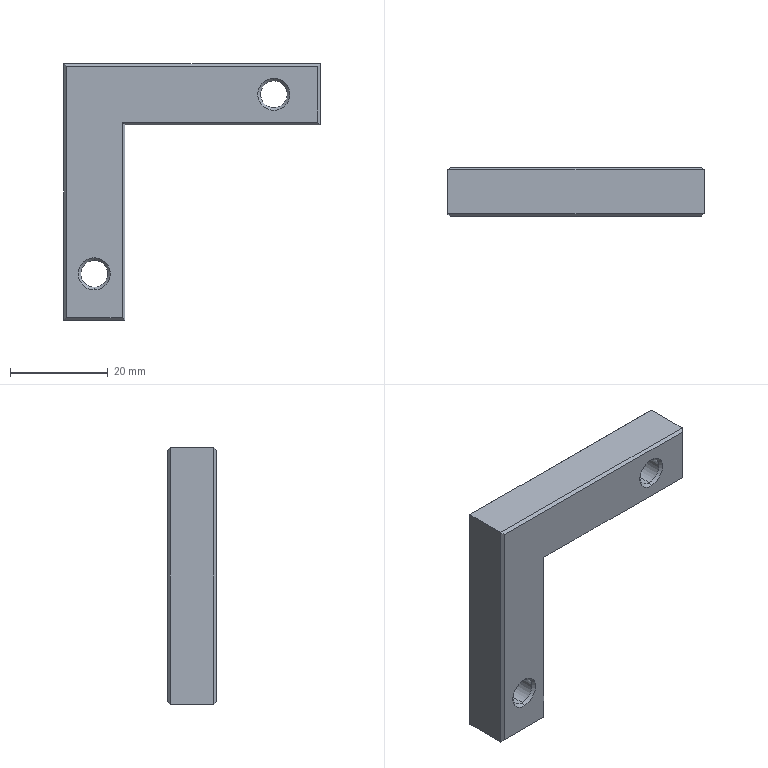Part | 1 solid | 38 faces | box 52.5 x 10 x 52.5 mm | volume 10387 mm3 | plane 22 | cone 8 | cylinder 8 | commonest cylinder face diameters 5.5 x4 10 x4
STEP:
#1=CARTESIAN_POINT('',(43.,9.46,-11.25));
#2=VERTEX_POINT('',#1);
#3=CARTESIAN_POINT('',(43.,9.46,-1.25));
#4=VERTEX_POINT('',#3);
#5=CARTESIAN_POINT('',(43.,9.46,-6.25));
#6=DIRECTION('',(0.,1.,0.));
#7=DIRECTION('',(0.,0.,-1.));
#8=AXIS2_PLACEMENT_3D('',#5,#6,#7);
#9=CIRCLE('',#8,5.);
#10=EDGE_CURVE('',#2,#4,#9,.T.);
#11=ORIENTED_EDGE('',*,*,#10,.F.);
#12=CARTESIAN_POINT('',(43.,10.,-11.79));
#13=VERTEX_POINT('',#12);
#14=CARTESIAN_POINT('',(43.,9.46,-11.25));
#15=DIRECTION('',(0.,0.7071,-0.7071));
#16=VECTOR('',#15,1000.);
#17=LINE('',#14,#16);
#18=EDGE_CURVE('',#2,#13,#17,.T.);
#19=ORIENTED_EDGE('',*,*,#18,.T.);
#20=CARTESIAN_POINT('',(43.,10.,-0.71));
#21=VERTEX_POINT('',#20);
#22=CARTESIAN_POINT('',(43.,10.,-6.25));
#23=DIRECTION('',(0.,-1.,0.));
#24=DIRECTION('',(0.,0.,-1.));
#25=AXIS2_PLACEMENT_3D('',#22,#23,#24);
#26=CIRCLE('',#25,5.54);
#27=EDGE_CURVE('',#21,#13,#26,.T.);
#28=ORIENTED_EDGE('',*,*,#27,.F.);
#29=CARTESIAN_POINT('',(43.,9.46,-1.25));
#30=DIRECTION('',(0.,0.7071,0.7071));
#31=VECTOR('',#30,1000.);
#32=LINE('',#29,#31);
#33=EDGE_CURVE('',#4,#21,#32,.T.);
#34=ORIENTED_EDGE('',*,*,#33,.F.);
#35=EDGE_LOOP('',(#11,#19,#28,#34));
#36=FACE_OUTER_BOUND('',#35,.T.);
#37=CARTESIAN_POINT('',(43.,9.46,-6.25));
#38=DIRECTION('',(0.,1.,0.));
#39=DIRECTION('',(0.,0.,1.));
#40=AXIS2_PLACEMENT_3D('',#37,#38,#39);
#41=CONICAL_SURFACE('',#40,5.,0.7854);
#42=ADVANCED_FACE('',(#36),#41,.F.);
#43=CARTESIAN_POINT('',(6.25,9.46,-48.));
#44=VERTEX_POINT('',#43);
#45=CARTESIAN_POINT('',(6.25,9.46,-38.));
#46=VERTEX_POINT('',#45);
#47=CARTESIAN_POINT('',(6.25,9.46,-43.));
#48=DIRECTION('',(0.,1.,0.));
#49=DIRECTION('',(0.,0.,-1.));
#50=AXIS2_PLACEMENT_3D('',#47,#48,#49);
#51=CIRCLE('',#50,5.);
#52=EDGE_CURVE('',#44,#46,#51,.T.);
#53=ORIENTED_EDGE('',*,*,#52,.F.);
#54=CARTESIAN_POINT('',(6.25,10.,-48.54));
#55=VERTEX_POINT('',#54);
#56=CARTESIAN_POINT('',(6.25,9.46,-48.));
#57=DIRECTION('',(0.,0.7071,-0.7071));
#58=VECTOR('',#57,1000.);
#59=LINE('',#56,#58);
#60=EDGE_CURVE('',#44,#55,#59,.T.);
#61=ORIENTED_EDGE('',*,*,#60,.T.);
#62=CARTESIAN_POINT('',(6.25,10.,-37.46));
#63=VERTEX_POINT('',#62);
#64=CARTESIAN_POINT('',(6.25,10.,-43.));
#65=DIRECTION('',(0.,-1.,0.));
#66=DIRECTION('',(0.,0.,-1.));
#67=AXIS2_PLACEMENT_3D('',#64,#65,#66);
#68=CIRCLE('',#67,5.54);
#69=EDGE_CURVE('',#63,#55,#68,.T.);
#70=ORIENTED_EDGE('',*,*,#69,.F.);
#71=CARTESIAN_POINT('',(6.25,9.46,-38.));
#72=DIRECTION('',(0.,0.7071,0.7071));
#73=VECTOR('',#72,1000.);
#74=LINE('',#71,#73);
#75=EDGE_CURVE('',#46,#63,#74,.T.);
#76=ORIENTED_EDGE('',*,*,#75,.F.);
#77=EDGE_LOOP('',(#53,#61,#70,#76));
#78=FACE_OUTER_BOUND('',#77,.T.);
#79=CARTESIAN_POINT('',(6.25,9.46,-43.));
#80=DIRECTION('',(0.,1.,0.));
#81=DIRECTION('',(0.,0.,1.));
#82=AXIS2_PLACEMENT_3D('',#79,#80,#81);
#83=CONICAL_SURFACE('',#82,5.,0.7854);
#84=ADVANCED_FACE('',(#78),#83,.F.);
#85=CARTESIAN_POINT('',(43.,0.54,-3.5));
#86=VERTEX_POINT('',#85);
#87=CARTESIAN_POINT('',(43.,0.54,-9.));
#88=VERTEX_POINT('',#87);
#89=CARTESIAN_POINT('',(43.,0.54,-6.25));
#90=DIRECTION('',(0.,-1.,0.));
#91=DIRECTION('',(0.,0.,-1.));
#92=AXIS2_PLACEMENT_3D('',#89,#90,#91);
#93=CIRCLE('',#92,2.75);
#94=EDGE_CURVE('',#86,#88,#93,.T.);
#95=ORIENTED_EDGE('',*,*,#94,.F.);
#96=CARTESIAN_POINT('',(43.,0.,-2.96));
#97=VERTEX_POINT('',#96);
#98=CARTESIAN_POINT('',(43.,0.,-2.96));
#99=DIRECTION('',(0.,-0.7071,0.7071));
#100=VECTOR('',#99,1000.);
#101=LINE('',#98,#100);
#102=EDGE_CURVE('',#86,#97,#101,.T.);
#103=ORIENTED_EDGE('',*,*,#102,.T.);
#104=CARTESIAN_POINT('',(43.,0.,-9.54));
#105=VERTEX_POINT('',#104);
#106=CARTESIAN_POINT('',(43.,0.,-6.25));
#107=DIRECTION('',(0.,1.,0.));
#108=DIRECTION('',(0.,0.,-1.));
#109=AXIS2_PLACEMENT_3D('',#106,#107,#108);
#110=CIRCLE('',#109,3.29);
#111=EDGE_CURVE('',#105,#97,#110,.T.);
#112=ORIENTED_EDGE('',*,*,#111,.F.);
#113=CARTESIAN_POINT('',(43.,0.,-9.54));
#114=DIRECTION('',(0.,-0.7071,-0.7071));
#115=VECTOR('',#114,1000.);
#116=LINE('',#113,#115);
#117=EDGE_CURVE('',#88,#105,#116,.T.);
#118=ORIENTED_EDGE('',*,*,#117,.F.);
#119=EDGE_LOOP('',(#95,#103,#112,#118));
#120=FACE_OUTER_BOUND('',#119,.T.);
#121=CARTESIAN_POINT('',(43.,0.,-6.25));
#122=DIRECTION('',(0.,-1.,0.));
#123=DIRECTION('',(0.,0.,-1.));
#124=AXIS2_PLACEMENT_3D('',#121,#122,#123);
#125=CONICAL_SURFACE('',#124,3.29,0.7854);
#126=ADVANCED_FACE('',(#120),#125,.F.);
#127=CARTESIAN_POINT('',(6.25,0.54,-40.25));
#128=VERTEX_POINT('',#127);
#129=CARTESIAN_POINT('',(6.25,0.54,-45.75));
#130=VERTEX_POINT('',#129);
#131=CARTESIAN_POINT('',(6.25,0.54,-43.));
#132=DIRECTION('',(0.,-1.,0.));
#133=DIRECTION('',(0.,0.,-1.));
#134=AXIS2_PLACEMENT_3D('',#131,#132,#133);
#135=CIRCLE('',#134,2.75);
#136=EDGE_CURVE('',#128,#130,#135,.T.);
#137=ORIENTED_EDGE('',*,*,#136,.F.);
#138=CARTESIAN_POINT('',(6.25,0.,-39.71));
#139=VERTEX_POINT('',#138);
#140=CARTESIAN_POINT('',(6.25,0.,-39.71));
#141=DIRECTION('',(0.,-0.7071,0.7071));
#142=VECTOR('',#141,1000.);
#143=LINE('',#140,#142);
#144=EDGE_CURVE('',#128,#139,#143,.T.);
#145=ORIENTED_EDGE('',*,*,#144,.T.);
#146=CARTESIAN_POINT('',(6.25,0.,-46.29));
#147=VERTEX_POINT('',#146);
#148=CARTESIAN_POINT('',(6.25,0.,-43.));
#149=DIRECTION('',(0.,1.,0.));
#150=DIRECTION('',(0.,0.,-1.));
#151=AXIS2_PLACEMENT_3D('',#148,#149,#150);
#152=CIRCLE('',#151,3.29);
#153=EDGE_CURVE('',#147,#139,#152,.T.);
#154=ORIENTED_EDGE('',*,*,#153,.F.);
#155=CARTESIAN_POINT('',(6.25,0.,-46.29));
#156=DIRECTION('',(0.,-0.7071,-0.7071));
#157=VECTOR('',#156,1000.);
#158=LINE('',#155,#157);
#159=EDGE_CURVE('',#130,#147,#158,.T.);
#160=ORIENTED_EDGE('',*,*,#159,.F.);
#161=EDGE_LOOP('',(#137,#145,#154,#160));
#162=FACE_OUTER_BOUND('',#161,.T.);
#163=CARTESIAN_POINT('',(6.25,0.,-43.));
#164=DIRECTION('',(0.,-1.,0.));
#165=DIRECTION('',(0.,0.,-1.));
#166=AXIS2_PLACEMENT_3D('',#163,#164,#165);
#167=CONICAL_SURFACE('',#166,3.29,0.7854);
#168=ADVANCED_FACE('',(#162),#167,.F.);
#169=CARTESIAN_POINT('',(43.,4.3,-11.25));
#170=VERTEX_POINT('',#169);
#171=CARTESIAN_POINT('',(43.,4.3,-1.25));
#172=VERTEX_POINT('',#171);
#173=CARTESIAN_POINT('',(43.,4.3,-6.25));
#174=DIRECTION('',(0.,1.,0.));
#175=DIRECTION('',(0.,0.,1.));
#176=AXIS2_PLACEMENT_3D('',#173,#174,#175);
#177=CIRCLE('',#176,5.);
#178=EDGE_CURVE('',#170,#172,#177,.T.);
#179=ORIENTED_EDGE('',*,*,#178,.F.);
#180=CARTESIAN_POINT('',(43.,10.,-11.25));
#181=DIRECTION('',(0.,1.,0.));
#182=VECTOR('',#181,1000.);
#183=LINE('',#180,#182);
#184=EDGE_CURVE('',#170,#2,#183,.T.);
#185=ORIENTED_EDGE('',*,*,#184,.T.);
#186=ORIENTED_EDGE('',*,*,#10,.T.);
#187=CARTESIAN_POINT('',(43.,10.,-1.25));
#188=DIRECTION('',(0.,1.,0.));
#189=VECTOR('',#188,1000.);
#190=LINE('',#187,#189);
#191=EDGE_CURVE('',#172,#4,#190,.T.);
#192=ORIENTED_EDGE('',*,*,#191,.F.);
#193=EDGE_LOOP('',(#179,#185,#186,#192));
#194=FACE_OUTER_BOUND('',#193,.T.);
#195=CARTESIAN_POINT('',(43.,10.,-6.25));
#196=DIRECTION('',(0.,1.,0.));
#197=DIRECTION('',(0.,0.,1.));
#198=AXIS2_PLACEMENT_3D('',#195,#196,#197);
#199=CYLINDRICAL_SURFACE('',#198,5.);
#200=ADVANCED_FACE('',(#194),#199,.F.);
#201=ORIENTED_EDGE('',*,*,#94,.T.);
#202=CARTESIAN_POINT('',(43.,4.3,-9.));
#203=VERTEX_POINT('',#202);
#204=CARTESIAN_POINT('',(43.,10.,-9.));
#205=DIRECTION('',(0.,1.,0.));
#206=VECTOR('',#205,1000.);
#207=LINE('',#204,#206);
#208=EDGE_CURVE('',#88,#203,#207,.T.);
#209=ORIENTED_EDGE('',*,*,#208,.T.);
#210=CARTESIAN_POINT('',(43.,4.3,-3.5));
#211=VERTEX_POINT('',#210);
#212=CARTESIAN_POINT('',(43.,4.3,-6.25));
#213=DIRECTION('',(0.,1.,0.));
#214=DIRECTION('',(0.,0.,1.));
#215=AXIS2_PLACEMENT_3D('',#212,#213,#214);
#216=CIRCLE('',#215,2.75);
#217=EDGE_CURVE('',#203,#211,#216,.T.);
#218=ORIENTED_EDGE('',*,*,#217,.T.);
#219=CARTESIAN_POINT('',(43.,10.,-3.5));
#220=DIRECTION('',(0.,1.,0.));
#221=VECTOR('',#220,1000.);
#222=LINE('',#219,#221);
#223=EDGE_CURVE('',#86,#211,#222,.T.);
#224=ORIENTED_EDGE('',*,*,#223,.F.);
#225=EDGE_LOOP('',(#201,#209,#218,#224));
#226=FACE_OUTER_BOUND('',#225,.T.);
#227=CARTESIAN_POINT('',(43.,10.,-6.25));
#228=DIRECTION('',(0.,1.,0.));
#229=DIRECTION('',(0.,0.,1.));
#230=AXIS2_PLACEMENT_3D('',#227,#228,#229);
#231=CYLINDRICAL_SURFACE('',#230,2.75);
#232=ADVANCED_FACE('',(#226),#231,.F.);
#233=CARTESIAN_POINT('',(6.25,4.3,-48.));
#234=VERTEX_POINT('',#233);
#235=CARTESIAN_POINT('',(6.25,4.3,-38.));
#236=VERTEX_POINT('',#235);
#237=CARTESIAN_POINT('',(6.25,4.3,-43.));
#238=DIRECTION('',(0.,1.,0.));
#239=DIRECTION('',(0.,0.,1.));
#240=AXIS2_PLACEMENT_3D('',#237,#238,#239);
#241=CIRCLE('',#240,5.);
#242=EDGE_CURVE('',#234,#236,#241,.T.);
#243=ORIENTED_EDGE('',*,*,#242,.F.);
#244=CARTESIAN_POINT('',(6.25,10.,-48.));
#245=DIRECTION('',(0.,1.,0.));
#246=VECTOR('',#245,1000.);
#247=LINE('',#244,#246);
#248=EDGE_CURVE('',#234,#44,#247,.T.);
#249=ORIENTED_EDGE('',*,*,#248,.T.);
#250=ORIENTED_EDGE('',*,*,#52,.T.);
#251=CARTESIAN_POINT('',(6.25,10.,-38.));
#252=DIRECTION('',(0.,1.,0.));
#253=VECTOR('',#252,1000.);
#254=LINE('',#251,#253);
#255=EDGE_CURVE('',#236,#46,#254,.T.);
#256=ORIENTED_EDGE('',*,*,#255,.F.);
#257=EDGE_LOOP('',(#243,#249,#250,#256));
#258=FACE_OUTER_BOUND('',#257,.T.);
#259=CARTESIAN_POINT('',(6.25,10.,-43.));
#260=DIRECTION('',(0.,1.,0.));
#261=DIRECTION('',(0.,0.,1.));
#262=AXIS2_PLACEMENT_3D('',#259,#260,#261);
#263=CYLINDRICAL_SURFACE('',#262,5.);
#264=ADVANCED_FACE('',(#258),#263,.F.);
#265=ORIENTED_EDGE('',*,*,#136,.T.);
#266=CARTESIAN_POINT('',(6.25,4.3,-45.75));
#267=VERTEX_POINT('',#266);
#268=CARTESIAN_POINT('',(6.25,10.,-45.75));
#269=DIRECTION('',(0.,1.,0.));
#270=VECTOR('',#269,1000.);
#271=LINE('',#268,#270);
#272=EDGE_CURVE('',#130,#267,#271,.T.);
#273=ORIENTED_EDGE('',*,*,#272,.T.);
#274=CARTESIAN_POINT('',(6.25,4.3,-40.25));
#275=VERTEX_POINT('',#274);
#276=CARTESIAN_POINT('',(6.25,4.3,-43.));
#277=DIRECTION('',(0.,1.,0.));
#278=DIRECTION('',(0.,0.,1.));
#279=AXIS2_PLACEMENT_3D('',#276,#277,#278);
#280=CIRCLE('',#279,2.75);
#281=EDGE_CURVE('',#267,#275,#280,.T.);
#282=ORIENTED_EDGE('',*,*,#281,.T.);
#283=CARTESIAN_POINT('',(6.25,10.,-40.25));
#284=DIRECTION('',(0.,1.,0.));
#285=VECTOR('',#284,1000.);
#286=LINE('',#283,#285);
#287=EDGE_CURVE('',#128,#275,#286,.T.);
#288=ORIENTED_EDGE('',*,*,#287,.F.);
#289=EDGE_LOOP('',(#265,#273,#282,#288));
#290=FACE_OUTER_BOUND('',#289,.T.);
#291=CARTESIAN_POINT('',(6.25,10.,-43.));
#292=DIRECTION('',(0.,1.,0.));
#293=DIRECTION('',(0.,0.,1.));
#294=AXIS2_PLACEMENT_3D('',#291,#292,#293);
#295=CYLINDRICAL_SURFACE('',#294,2.75);
#296=ADVANCED_FACE('',(#290),#295,.F.);
#297=CARTESIAN_POINT('',(0.,9.46,0.));
#298=VERTEX_POINT('',#297);
#299=CARTESIAN_POINT('',(0.,0.54,0.));
#300=VERTEX_POINT('',#299);
#301=CARTESIAN_POINT('',(0.,10.,0.));
#302=DIRECTION('',(0.,-1.,0.));
#303=VECTOR('',#302,1000.);
#304=LINE('',#301,#303);
#305=EDGE_CURVE('',#298,#300,#304,.T.);
#306=ORIENTED_EDGE('',*,*,#305,.T.);
#307=CARTESIAN_POINT('',(52.5,0.54,0.));
#308=VERTEX_POINT('',#307);
#309=CARTESIAN_POINT('',(52.5,0.54,0.));
#310=DIRECTION('',(1.,0.,0.));
#311=VECTOR('',#310,1000.);
#312=LINE('',#309,#311);
#313=EDGE_CURVE('',#300,#308,#312,.T.);
#314=ORIENTED_EDGE('',*,*,#313,.T.);
#315=CARTESIAN_POINT('',(52.5,9.46,0.));
#316=VERTEX_POINT('',#315);
#317=CARTESIAN_POINT('',(52.5,10.,0.));
#318=DIRECTION('',(0.,-1.,0.));
#319=VECTOR('',#318,1000.);
#320=LINE('',#317,#319);
#321=EDGE_CURVE('',#316,#308,#320,.T.);
#322=ORIENTED_EDGE('',*,*,#321,.F.);
#323=CARTESIAN_POINT('',(52.5,9.46,0.));
#324=DIRECTION('',(-1.,0.,0.));
#325=VECTOR('',#324,1000.);
#326=LINE('',#323,#325);
#327=EDGE_CURVE('',#316,#298,#326,.T.);
#328=ORIENTED_EDGE('',*,*,#327,.T.);
#329=EDGE_LOOP('',(#306,#314,#322,#328));
#330=FACE_OUTER_BOUND('',#329,.T.);
#331=CARTESIAN_POINT('',(52.5,10.,0.));
#332=DIRECTION('',(0.,0.,-1.));
#333=DIRECTION('',(-1.,0.,0.));
#334=AXIS2_PLACEMENT_3D('',#331,#332,#333);
#335=PLANE('',#334);
#336=ADVANCED_FACE('',(#330),#335,.F.);
#337=ORIENTED_EDGE('',*,*,#321,.T.);
#338=CARTESIAN_POINT('',(52.5,0.54,-12.5));
#339=VERTEX_POINT('',#338);
#340=CARTESIAN_POINT('',(52.5,0.54,-12.5));
#341=DIRECTION('',(0.,0.,-1.));
#342=VECTOR('',#341,1000.);
#343=LINE('',#340,#342);
#344=EDGE_CURVE('',#308,#339,#343,.T.);
#345=ORIENTED_EDGE('',*,*,#344,.T.);
#346=CARTESIAN_POINT('',(52.5,9.46,-12.5));
#347=VERTEX_POINT('',#346);
#348=CARTESIAN_POINT('',(52.5,10.,-12.5));
#349=DIRECTION('',(0.,-1.,0.));
#350=VECTOR('',#349,1000.);
#351=LINE('',#348,#350);
#352=EDGE_CURVE('',#347,#339,#351,.T.);
#353=ORIENTED_EDGE('',*,*,#352,.F.);
#354=CARTESIAN_POINT('',(52.5,9.46,-12.5));
#355=DIRECTION('',(0.,0.,1.));
#356=VECTOR('',#355,1000.);
#357=LINE('',#354,#356);
#358=EDGE_CURVE('',#347,#316,#357,.T.);
#359=ORIENTED_EDGE('',*,*,#358,.T.);
#360=EDGE_LOOP('',(#337,#345,#353,#359));
#361=FACE_OUTER_BOUND('',#360,.T.);
#362=CARTESIAN_POINT('',(52.5,10.,-12.5));
#363=DIRECTION('',(-1.,0.,0.));
#364=DIRECTION('',(0.,0.,1.));
#365=AXIS2_PLACEMENT_3D('',#362,#363,#364);
#366=PLANE('',#365);
#367=ADVANCED_FACE('',(#361),#366,.F.);
#368=ORIENTED_EDGE('',*,*,#352,.T.);
#369=CARTESIAN_POINT('',(12.5,0.54,-12.5));
#370=VERTEX_POINT('',#369);
#371=CARTESIAN_POINT('',(12.5,0.54,-12.5));
#372=DIRECTION('',(-1.,0.,0.));
#373=VECTOR('',#372,1000.);
#374=LINE('',#371,#373);
#375=EDGE_CURVE('',#339,#370,#374,.T.);
#376=ORIENTED_EDGE('',*,*,#375,.T.);
#377=CARTESIAN_POINT('',(12.5,9.46,-12.5));
#378=VERTEX_POINT('',#377);
#379=CARTESIAN_POINT('',(12.5,10.,-12.5));
#380=DIRECTION('',(0.,-1.,0.));
#381=VECTOR('',#380,1000.);
#382=LINE('',#379,#381);
#383=EDGE_CURVE('',#378,#370,#382,.T.);
#384=ORIENTED_EDGE('',*,*,#383,.F.);
#385=CARTESIAN_POINT('',(12.5,9.46,-12.5));
#386=DIRECTION('',(1.,0.,0.));
#387=VECTOR('',#386,1000.);
#388=LINE('',#385,#387);
#389=EDGE_CURVE('',#378,#347,#388,.T.);
#390=ORIENTED_EDGE('',*,*,#389,.T.);
#391=EDGE_LOOP('',(#368,#376,#384,#390));
#392=FACE_OUTER_BOUND('',#391,.T.);
#393=CARTESIAN_POINT('',(12.5,10.,-12.5));
#394=DIRECTION('',(0.,0.,1.));
#395=DIRECTION('',(1.,0.,0.));
#396=AXIS2_PLACEMENT_3D('',#393,#394,#395);
#397=PLANE('',#396);
#398=ADVANCED_FACE('',(#392),#397,.F.);
#399=ORIENTED_EDGE('',*,*,#383,.T.);
#400=CARTESIAN_POINT('',(12.5,0.54,-52.5));
#401=VERTEX_POINT('',#400);
#402=CARTESIAN_POINT('',(12.5,0.54,-52.5));
#403=DIRECTION('',(0.,0.,-1.));
#404=VECTOR('',#403,1000.);
#405=LINE('',#402,#404);
#406=EDGE_CURVE('',#370,#401,#405,.T.);
#407=ORIENTED_EDGE('',*,*,#406,.T.);
#408=CARTESIAN_POINT('',(12.5,9.46,-52.5));
#409=VERTEX_POINT('',#408);
#410=CARTESIAN_POINT('',(12.5,10.,-52.5));
#411=DIRECTION('',(0.,-1.,0.));
#412=VECTOR('',#411,1000.);
#413=LINE('',#410,#412);
#414=EDGE_CURVE('',#409,#401,#413,.T.);
#415=ORIENTED_EDGE('',*,*,#414,.F.);
#416=CARTESIAN_POINT('',(12.5,9.46,-52.5));
#417=DIRECTION('',(0.,0.,1.));
#418=VECTOR('',#417,1000.);
#419=LINE('',#416,#418);
#420=EDGE_CURVE('',#409,#378,#419,.T.);
#421=ORIENTED_EDGE('',*,*,#420,.T.);
#422=EDGE_LOOP('',(#399,#407,#415,#421));
#423=FACE_OUTER_BOUND('',#422,.T.);
#424=CARTESIAN_POINT('',(12.5,10.,-52.5));
#425=DIRECTION('',(-1.,0.,0.));
#426=DIRECTION('',(0.,0.,1.));
#427=AXIS2_PLACEMENT_3D('',#424,#425,#426);
#428=PLANE('',#427);
#429=ADVANCED_FACE('',(#423),#428,.F.);
#430=ORIENTED_EDGE('',*,*,#414,.T.);
#431=CARTESIAN_POINT('',(0.,0.54,-52.5));
#432=VERTEX_POINT('',#431);
#433=CARTESIAN_POINT('',(0.,0.54,-52.5));
#434=DIRECTION('',(-1.,0.,0.));
#435=VECTOR('',#434,1000.);
#436=LINE('',#433,#435);
#437=EDGE_CURVE('',#401,#432,#436,.T.);
#438=ORIENTED_EDGE('',*,*,#437,.T.);
#439=CARTESIAN_POINT('',(0.,9.46,-52.5));
#440=VERTEX_POINT('',#439);
#441=CARTESIAN_POINT('',(0.,10.,-52.5));
#442=DIRECTION('',(0.,-1.,0.));
#443=VECTOR('',#442,1000.);
#444=LINE('',#441,#443);
#445=EDGE_CURVE('',#440,#432,#444,.T.);
#446=ORIENTED_EDGE('',*,*,#445,.F.);
#447=CARTESIAN_POINT('',(0.,9.46,-52.5));
#448=DIRECTION('',(1.,0.,0.));
#449=VECTOR('',#448,1000.);
#450=LINE('',#447,#449);
#451=EDGE_CURVE('',#440,#409,#450,.T.);
#452=ORIENTED_EDGE('',*,*,#451,.T.);
#453=EDGE_LOOP('',(#430,#438,#446,#452));
#454=FACE_OUTER_BOUND('',#453,.T.);
#455=CARTESIAN_POINT('',(0.,10.,-52.5));
#456=DIRECTION('',(0.,0.,1.));
#457=DIRECTION('',(1.,0.,0.));
#458=AXIS2_PLACEMENT_3D('',#455,#456,#457);
#459=PLANE('',#458);
#460=ADVANCED_FACE('',(#454),#459,.F.);
#461=ORIENTED_EDGE('',*,*,#445,.T.);
#462=CARTESIAN_POINT('',(0.,0.54,0.));
#463=DIRECTION('',(0.,0.,1.));
#464=VECTOR('',#463,1000.);
#465=LINE('',#462,#464);
#466=EDGE_CURVE('',#432,#300,#465,.T.);
#467=ORIENTED_EDGE('',*,*,#466,.T.);
#468=ORIENTED_EDGE('',*,*,#305,.F.);
#469=CARTESIAN_POINT('',(0.,9.46,0.));
#470=DIRECTION('',(0.,0.,-1.));
#471=VECTOR('',#470,1000.);
#472=LINE('',#469,#471);
#473=EDGE_CURVE('',#298,#440,#472,.T.);
#474=ORIENTED_EDGE('',*,*,#473,.T.);
#475=EDGE_LOOP('',(#461,#467,#468,#474));
#476=FACE_OUTER_BOUND('',#475,.T.);
#477=CARTESIAN_POINT('',(0.,10.,0.));
#478=DIRECTION('',(1.,0.,0.));
#479=DIRECTION('',(0.,0.,-1.));
#480=AXIS2_PLACEMENT_3D('',#477,#478,#479);
#481=PLANE('',#480);
#482=ADVANCED_FACE('',(#476),#481,.F.);
#483=CARTESIAN_POINT('',(11.96,10.,-51.96));
#484=VERTEX_POINT('',#483);
#485=CARTESIAN_POINT('',(0.54,10.,-51.96));
#486=VERTEX_POINT('',#485);
#487=CARTESIAN_POINT('',(0.,10.,-51.96));
#488=DIRECTION('',(-1.,0.,0.));
#489=VECTOR('',#488,1000.);
#490=LINE('',#487,#489);
#491=EDGE_CURVE('',#484,#486,#490,.T.);
#492=ORIENTED_EDGE('',*,*,#491,.T.);
#493=CARTESIAN_POINT('',(0.54,10.,-0.54));
#494=VERTEX_POINT('',#493);
#495=CARTESIAN_POINT('',(0.54,10.,0.));
#496=DIRECTION('',(0.,0.,1.));
#497=VECTOR('',#496,1000.);
#498=LINE('',#495,#497);
#499=EDGE_CURVE('',#486,#494,#498,.T.);
#500=ORIENTED_EDGE('',*,*,#499,.T.);
#501=CARTESIAN_POINT('',(51.96,10.,-0.54));
#502=VERTEX_POINT('',#501);
#503=CARTESIAN_POINT('',(0.,10.,-0.54));
#504=DIRECTION('',(1.,0.,0.));
#505=VECTOR('',#504,1000.);
#506=LINE('',#503,#505);
#507=EDGE_CURVE('',#494,#502,#506,.T.);
#508=ORIENTED_EDGE('',*,*,#507,.T.);
#509=CARTESIAN_POINT('',(51.96,10.,-11.96));
#510=VERTEX_POINT('',#509);
#511=CARTESIAN_POINT('',(51.96,10.,0.));
#512=DIRECTION('',(0.,0.,-1.));
#513=VECTOR('',#512,1000.);
#514=LINE('',#511,#513);
#515=EDGE_CURVE('',#502,#510,#514,.T.);
#516=ORIENTED_EDGE('',*,*,#515,.T.);
#517=CARTESIAN_POINT('',(11.96,10.,-11.96));
#518=VERTEX_POINT('',#517);
#519=CARTESIAN_POINT('',(0.,10.,-11.96));
#520=DIRECTION('',(-1.,0.,0.));
#521=VECTOR('',#520,1000.);
#522=LINE('',#519,#521);
#523=EDGE_CURVE('',#510,#518,#522,.T.);
#524=ORIENTED_EDGE('',*,*,#523,.T.);
#525=CARTESIAN_POINT('',(11.96,10.,0.));
#526=DIRECTION('',(0.,0.,-1.));
#527=VECTOR('',#526,1000.);
#528=LINE('',#525,#527);
#529=EDGE_CURVE('',#518,#484,#528,.T.);
#530=ORIENTED_EDGE('',*,*,#529,.T.);
#531=EDGE_LOOP('',(#492,#500,#508,#516,#524,#530));
#532=FACE_OUTER_BOUND('',#531,.T.);
#533=ORIENTED_EDGE('',*,*,#69,.T.);
#534=CARTESIAN_POINT('',(6.25,10.,-43.));
#535=DIRECTION('',(0.,-1.,0.));
#536=DIRECTION('',(0.,0.,-1.));
#537=AXIS2_PLACEMENT_3D('',#534,#535,#536);
#538=CIRCLE('',#537,5.54);
#539=EDGE_CURVE('',#55,#63,#538,.T.);
#540=ORIENTED_EDGE('',*,*,#539,.T.);
#541=EDGE_LOOP('',(#533,#540));
#542=FACE_BOUND('',#541,.T.);
#543=ORIENTED_EDGE('',*,*,#27,.T.);
#544=CARTESIAN_POINT('',(43.,10.,-6.25));
#545=DIRECTION('',(0.,-1.,0.));
#546=DIRECTION('',(0.,0.,-1.));
#547=AXIS2_PLACEMENT_3D('',#544,#545,#546);
#548=CIRCLE('',#547,5.54);
#549=EDGE_CURVE('',#13,#21,#548,.T.);
#550=ORIENTED_EDGE('',*,*,#549,.T.);
#551=EDGE_LOOP('',(#543,#550));
#552=FACE_BOUND('',#551,.T.);
#553=CARTESIAN_POINT('',(0.,10.,0.));
#554=DIRECTION('',(0.,-1.,0.));
#555=DIRECTION('',(0.,0.,-1.));
#556=AXIS2_PLACEMENT_3D('',#553,#554,#555);
#557=PLANE('',#556);
#558=ADVANCED_FACE('',(#532,#542,#552),#557,.F.);
#559=CARTESIAN_POINT('',(11.96,0.,-11.96));
#560=VERTEX_POINT('',#559);
#561=CARTESIAN_POINT('',(51.96,0.,-11.96));
#562=VERTEX_POINT('',#561);
#563=CARTESIAN_POINT('',(52.5,0.,-11.96));
#564=DIRECTION('',(1.,0.,0.));
#565=VECTOR('',#564,1000.);
#566=LINE('',#563,#565);
#567=EDGE_CURVE('',#560,#562,#566,.T.);
#568=ORIENTED_EDGE('',*,*,#567,.T.);
#569=CARTESIAN_POINT('',(51.96,0.,-0.54));
#570=VERTEX_POINT('',#569);
#571=CARTESIAN_POINT('',(51.96,0.,0.));
#572=DIRECTION('',(0.,0.,1.));
#573=VECTOR('',#572,1000.);
#574=LINE('',#571,#573);
#575=EDGE_CURVE('',#562,#570,#574,.T.);
#576=ORIENTED_EDGE('',*,*,#575,.T.);
#577=CARTESIAN_POINT('',(0.54,0.,-0.54));
#578=VERTEX_POINT('',#577);
#579=CARTESIAN_POINT('',(0.,0.,-0.54));
#580=DIRECTION('',(-1.,0.,0.));
#581=VECTOR('',#580,1000.);
#582=LINE('',#579,#581);
#583=EDGE_CURVE('',#570,#578,#582,.T.);
#584=ORIENTED_EDGE('',*,*,#583,.T.);
#585=CARTESIAN_POINT('',(0.54,0.,-51.96));
#586=VERTEX_POINT('',#585);
#587=CARTESIAN_POINT('',(0.54,0.,-52.5));
#588=DIRECTION('',(0.,0.,-1.));
#589=VECTOR('',#588,1000.);
#590=LINE('',#587,#589);
#591=EDGE_CURVE('',#578,#586,#590,.T.);
#592=ORIENTED_EDGE('',*,*,#591,.T.);
#593=CARTESIAN_POINT('',(11.96,0.,-51.96));
#594=VERTEX_POINT('',#593);
#595=CARTESIAN_POINT('',(12.5,0.,-51.96));
#596=DIRECTION('',(1.,0.,0.));
#597=VECTOR('',#596,1000.);
#598=LINE('',#595,#597);
#599=EDGE_CURVE('',#586,#594,#598,.T.);
#600=ORIENTED_EDGE('',*,*,#599,.T.);
#601=CARTESIAN_POINT('',(11.96,0.,-12.5));
#602=DIRECTION('',(0.,0.,1.));
#603=VECTOR('',#602,1000.);
#604=LINE('',#601,#603);
#605=EDGE_CURVE('',#594,#560,#604,.T.);
#606=ORIENTED_EDGE('',*,*,#605,.T.);
#607=EDGE_LOOP('',(#568,#576,#584,#592,#600,#606));
#608=FACE_OUTER_BOUND('',#607,.T.);
#609=ORIENTED_EDGE('',*,*,#153,.T.);
#610=CARTESIAN_POINT('',(6.25,0.,-43.));
#611=DIRECTION('',(0.,1.,0.));
#612=DIRECTION('',(0.,0.,-1.));
#613=AXIS2_PLACEMENT_3D('',#610,#611,#612);
#614=CIRCLE('',#613,3.29);
#615=EDGE_CURVE('',#139,#147,#614,.T.);
#616=ORIENTED_EDGE('',*,*,#615,.T.);
#617=EDGE_LOOP('',(#609,#616));
#618=FACE_BOUND('',#617,.T.);
#619=ORIENTED_EDGE('',*,*,#111,.T.);
#620=CARTESIAN_POINT('',(43.,0.,-6.25));
#621=DIRECTION('',(0.,1.,0.));
#622=DIRECTION('',(0.,0.,-1.));
#623=AXIS2_PLACEMENT_3D('',#620,#621,#622);
#624=CIRCLE('',#623,3.29);
#625=EDGE_CURVE('',#97,#105,#624,.T.);
#626=ORIENTED_EDGE('',*,*,#625,.T.);
#627=EDGE_LOOP('',(#619,#626));
#628=FACE_BOUND('',#627,.T.);
#629=CARTESIAN_POINT('',(0.,0.,0.));
#630=DIRECTION('',(0.,-1.,0.));
#631=DIRECTION('',(0.,0.,-1.));
#632=AXIS2_PLACEMENT_3D('',#629,#630,#631);
#633=PLANE('',#632);
#634=ADVANCED_FACE('',(#608,#618,#628),#633,.T.);
#635=ORIENTED_EDGE('',*,*,#272,.F.);
#636=CARTESIAN_POINT('',(6.25,0.54,-43.));
#637=DIRECTION('',(0.,-1.,0.));
#638=DIRECTION('',(0.,0.,-1.));
#639=AXIS2_PLACEMENT_3D('',#636,#637,#638);
#640=CIRCLE('',#639,2.75);
#641=EDGE_CURVE('',#130,#128,#640,.T.);
#642=ORIENTED_EDGE('',*,*,#641,.T.);
#643=ORIENTED_EDGE('',*,*,#287,.T.);
#644=CARTESIAN_POINT('',(6.25,4.3,-43.));
#645=DIRECTION('',(0.,1.,0.));
#646=DIRECTION('',(0.,0.,1.));
#647=AXIS2_PLACEMENT_3D('',#644,#645,#646);
#648=CIRCLE('',#647,2.75);
#649=EDGE_CURVE('',#275,#267,#648,.T.);
#650=ORIENTED_EDGE('',*,*,#649,.T.);
#651=EDGE_LOOP('',(#635,#642,#643,#650));
#652=FACE_OUTER_BOUND('',#651,.T.);
#653=CARTESIAN_POINT('',(6.25,10.,-43.));
#654=DIRECTION('',(0.,1.,0.));
#655=DIRECTION('',(0.,0.,1.));
#656=AXIS2_PLACEMENT_3D('',#653,#654,#655);
#657=CYLINDRICAL_SURFACE('',#656,2.75);
#658=ADVANCED_FACE('',(#652),#657,.F.);
#659=ORIENTED_EDGE('',*,*,#649,.F.);
#660=ORIENTED_EDGE('',*,*,#281,.F.);
#661=EDGE_LOOP('',(#659,#660));
#662=FACE_BOUND('',#661,.T.);
#663=CARTESIAN_POINT('',(6.25,4.3,-43.));
#664=DIRECTION('',(0.,1.,0.));
#665=DIRECTION('',(0.,0.,1.));
#666=AXIS2_PLACEMENT_3D('',#663,#664,#665);
#667=CIRCLE('',#666,5.);
#668=EDGE_CURVE('',#236,#234,#667,.T.);
#669=ORIENTED_EDGE('',*,*,#668,.T.);
#670=ORIENTED_EDGE('',*,*,#242,.T.);
#671=EDGE_LOOP('',(#669,#670));
#672=FACE_OUTER_BOUND('',#671,.T.);
#673=CARTESIAN_POINT('',(9.,4.3,-43.));
#674=DIRECTION('',(0.,-1.,0.));
#675=DIRECTION('',(0.,0.,-1.));
#676=AXIS2_PLACEMENT_3D('',#673,#674,#675);
#677=PLANE('',#676);
#678=ADVANCED_FACE('',(#662,#672),#677,.F.);
#679=ORIENTED_EDGE('',*,*,#248,.F.);
#680=ORIENTED_EDGE('',*,*,#668,.F.);
#681=ORIENTED_EDGE('',*,*,#255,.T.);
#682=CARTESIAN_POINT('',(6.25,9.46,-43.));
#683=DIRECTION('',(0.,1.,0.));
#684=DIRECTION('',(0.,0.,-1.));
#685=AXIS2_PLACEMENT_3D('',#682,#683,#684);
#686=CIRCLE('',#685,5.);
#687=EDGE_CURVE('',#46,#44,#686,.T.);
#688=ORIENTED_EDGE('',*,*,#687,.T.);
#689=EDGE_LOOP('',(#679,#680,#681,#688));
#690=FACE_OUTER_BOUND('',#689,.T.);
#691=CARTESIAN_POINT('',(6.25,10.,-43.));
#692=DIRECTION('',(0.,1.,0.));
#693=DIRECTION('',(0.,0.,1.));
#694=AXIS2_PLACEMENT_3D('',#691,#692,#693);
#695=CYLINDRICAL_SURFACE('',#694,5.);
#696=ADVANCED_FACE('',(#690),#695,.F.);
#697=ORIENTED_EDGE('',*,*,#208,.F.);
#698=CARTESIAN_POINT('',(43.,0.54,-6.25));
#699=DIRECTION('',(0.,-1.,0.));
#700=DIRECTION('',(0.,0.,-1.));
#701=AXIS2_PLACEMENT_3D('',#698,#699,#700);
#702=CIRCLE('',#701,2.75);
#703=EDGE_CURVE('',#88,#86,#702,.T.);
#704=ORIENTED_EDGE('',*,*,#703,.T.);
#705=ORIENTED_EDGE('',*,*,#223,.T.);
#706=CARTESIAN_POINT('',(43.,4.3,-6.25));
#707=DIRECTION('',(0.,1.,0.));
#708=DIRECTION('',(0.,0.,1.));
#709=AXIS2_PLACEMENT_3D('',#706,#707,#708);
#710=CIRCLE('',#709,2.75);
#711=EDGE_CURVE('',#211,#203,#710,.T.);
#712=ORIENTED_EDGE('',*,*,#711,.T.);
#713=EDGE_LOOP('',(#697,#704,#705,#712));
#714=FACE_OUTER_BOUND('',#713,.T.);
#715=CARTESIAN_POINT('',(43.,10.,-6.25));
#716=DIRECTION('',(0.,1.,0.));
#717=DIRECTION('',(0.,0.,1.));
#718=AXIS2_PLACEMENT_3D('',#715,#716,#717);
#719=CYLINDRICAL_SURFACE('',#718,2.75);
#720=ADVANCED_FACE('',(#714),#719,.F.);
#721=ORIENTED_EDGE('',*,*,#711,.F.);
#722=ORIENTED_EDGE('',*,*,#217,.F.);
#723=EDGE_LOOP('',(#721,#722));
#724=FACE_BOUND('',#723,.T.);
#725=CARTESIAN_POINT('',(43.,4.3,-6.25));
#726=DIRECTION('',(0.,1.,0.));
#727=DIRECTION('',(0.,0.,1.));
#728=AXIS2_PLACEMENT_3D('',#725,#726,#727);
#729=CIRCLE('',#728,5.);
#730=EDGE_CURVE('',#172,#170,#729,.T.);
#731=ORIENTED_EDGE('',*,*,#730,.T.);
#732=ORIENTED_EDGE('',*,*,#178,.T.);
#733=EDGE_LOOP('',(#731,#732));
#734=FACE_OUTER_BOUND('',#733,.T.);
#735=CARTESIAN_POINT('',(45.75,4.3,-6.25));
#736=DIRECTION('',(0.,-1.,0.));
#737=DIRECTION('',(0.,0.,-1.));
#738=AXIS2_PLACEMENT_3D('',#735,#736,#737);
#739=PLANE('',#738);
#740=ADVANCED_FACE('',(#724,#734),#739,.F.);
#741=ORIENTED_EDGE('',*,*,#184,.F.);
#742=ORIENTED_EDGE('',*,*,#730,.F.);
#743=ORIENTED_EDGE('',*,*,#191,.T.);
#744=CARTESIAN_POINT('',(43.,9.46,-6.25));
#745=DIRECTION('',(0.,1.,0.));
#746=DIRECTION('',(0.,0.,-1.));
#747=AXIS2_PLACEMENT_3D('',#744,#745,#746);
#748=CIRCLE('',#747,5.);
#749=EDGE_CURVE('',#4,#2,#748,.T.);
#750=ORIENTED_EDGE('',*,*,#749,.T.);
#751=EDGE_LOOP('',(#741,#742,#743,#750));
#752=FACE_OUTER_BOUND('',#751,.T.);
#753=CARTESIAN_POINT('',(43.,10.,-6.25));
#754=DIRECTION('',(0.,1.,0.));
#755=DIRECTION('',(0.,0.,1.));
#756=AXIS2_PLACEMENT_3D('',#753,#754,#755);
#757=CYLINDRICAL_SURFACE('',#756,5.);
#758=ADVANCED_FACE('',(#752),#757,.F.);
#759=CARTESIAN_POINT('',(8.333,-3.627,-48.333));
#760=DIRECTION('',(0.5774,0.5774,-0.5774));
#761=VECTOR('',#760,1000.);
#762=LINE('',#759,#761);
#763=EDGE_CURVE('',#594,#401,#762,.T.);
#764=ORIENTED_EDGE('',*,*,#763,.F.);
#765=ORIENTED_EDGE('',*,*,#599,.F.);
#766=CARTESIAN_POINT('',(17.5,-16.96,-35.));
#767=DIRECTION('',(0.5774,-0.5774,0.5774));
#768=VECTOR('',#767,1000.);
#769=LINE('',#766,#768);
#770=EDGE_CURVE('',#432,#586,#769,.T.);
#771=ORIENTED_EDGE('',*,*,#770,.F.);
#772=ORIENTED_EDGE('',*,*,#437,.F.);
#773=EDGE_LOOP('',(#764,#765,#771,#772));
#774=FACE_OUTER_BOUND('',#773,.T.);
#775=CARTESIAN_POINT('',(0.,0.54,-52.5));
#776=DIRECTION('',(0.,-0.7071,-0.7071));
#777=DIRECTION('',(1.,0.,0.));
#778=AXIS2_PLACEMENT_3D('',#775,#776,#777);
#779=PLANE('',#778);
#780=ADVANCED_FACE('',(#774),#779,.T.);
#781=ORIENTED_EDGE('',*,*,#770,.T.);
#782=ORIENTED_EDGE('',*,*,#591,.F.);
#783=CARTESIAN_POINT('',(17.5,-16.96,-17.5));
#784=DIRECTION('',(0.5774,-0.5774,-0.5774));
#785=VECTOR('',#784,1000.);
#786=LINE('',#783,#785);
#787=EDGE_CURVE('',#300,#578,#786,.T.);
#788=ORIENTED_EDGE('',*,*,#787,.F.);
#789=ORIENTED_EDGE('',*,*,#466,.F.);
#790=EDGE_LOOP('',(#781,#782,#788,#789));
#791=FACE_OUTER_BOUND('',#790,.T.);
#792=CARTESIAN_POINT('',(0.,0.54,0.));
#793=DIRECTION('',(-0.7071,-0.7071,0.));
#794=DIRECTION('',(0.,0.,-1.));
#795=AXIS2_PLACEMENT_3D('',#792,#793,#794);
#796=PLANE('',#795);
#797=ADVANCED_FACE('',(#791),#796,.T.);
#798=ORIENTED_EDGE('',*,*,#763,.T.);
#799=ORIENTED_EDGE('',*,*,#406,.F.);
#800=CARTESIAN_POINT('',(12.5,0.54,-12.5));
#801=DIRECTION('',(0.5774,0.5774,-0.5774));
#802=VECTOR('',#801,1000.);
#803=LINE('',#800,#802);
#804=EDGE_CURVE('',#560,#370,#803,.T.);
#805=ORIENTED_EDGE('',*,*,#804,.F.);
#806=ORIENTED_EDGE('',*,*,#605,.F.);
#807=EDGE_LOOP('',(#798,#799,#805,#806));
#808=FACE_OUTER_BOUND('',#807,.T.);
#809=CARTESIAN_POINT('',(12.5,0.54,-52.5));
#810=DIRECTION('',(0.7071,-0.7071,0.));
#811=DIRECTION('',(0.,0.,1.));
#812=AXIS2_PLACEMENT_3D('',#809,#810,#811);
#813=PLANE('',#812);
#814=ADVANCED_FACE('',(#808),#813,.T.);
#815=ORIENTED_EDGE('',*,*,#787,.T.);
#816=ORIENTED_EDGE('',*,*,#583,.F.);
#817=CARTESIAN_POINT('',(52.5,0.54,0.));
#818=DIRECTION('',(-0.5774,-0.5774,-0.5774));
#819=VECTOR('',#818,1000.);
#820=LINE('',#817,#819);
#821=EDGE_CURVE('',#308,#570,#820,.T.);
#822=ORIENTED_EDGE('',*,*,#821,.F.);
#823=ORIENTED_EDGE('',*,*,#313,.F.);
#824=EDGE_LOOP('',(#815,#816,#822,#823));
#825=FACE_OUTER_BOUND('',#824,.T.);
#826=CARTESIAN_POINT('',(52.5,0.54,0.));
#827=DIRECTION('',(0.,-0.7071,0.7071));
#828=DIRECTION('',(-1.,0.,0.));
#829=AXIS2_PLACEMENT_3D('',#826,#827,#828);
#830=PLANE('',#829);
#831=ADVANCED_FACE('',(#825),#830,.T.);
#832=ORIENTED_EDGE('',*,*,#804,.T.);
#833=ORIENTED_EDGE('',*,*,#375,.F.);
#834=CARTESIAN_POINT('',(39.167,-12.793,0.8333));
#835=DIRECTION('',(0.5774,0.5774,-0.5774));
#836=VECTOR('',#835,1000.);
#837=LINE('',#834,#836);
#838=EDGE_CURVE('',#562,#339,#837,.T.);
#839=ORIENTED_EDGE('',*,*,#838,.F.);
#840=ORIENTED_EDGE('',*,*,#567,.F.);
#841=EDGE_LOOP('',(#832,#833,#839,#840));
#842=FACE_OUTER_BOUND('',#841,.T.);
#843=CARTESIAN_POINT('',(12.5,0.54,-12.5));
#844=DIRECTION('',(0.,-0.7071,-0.7071));
#845=DIRECTION('',(1.,0.,0.));
#846=AXIS2_PLACEMENT_3D('',#843,#844,#845);
#847=PLANE('',#846);
#848=ADVANCED_FACE('',(#842),#847,.T.);
#849=ORIENTED_EDGE('',*,*,#821,.T.);
#850=ORIENTED_EDGE('',*,*,#575,.F.);
#851=ORIENTED_EDGE('',*,*,#838,.T.);
#852=ORIENTED_EDGE('',*,*,#344,.F.);
#853=EDGE_LOOP('',(#849,#850,#851,#852));
#854=FACE_OUTER_BOUND('',#853,.T.);
#855=CARTESIAN_POINT('',(52.5,0.54,-12.5));
#856=DIRECTION('',(0.7071,-0.7071,0.));
#857=DIRECTION('',(0.,0.,1.));
#858=AXIS2_PLACEMENT_3D('',#855,#856,#857);
#859=PLANE('',#858);
#860=ADVANCED_FACE('',(#854),#859,.T.);
#861=ORIENTED_EDGE('',*,*,#144,.F.);
#862=ORIENTED_EDGE('',*,*,#641,.F.);
#863=ORIENTED_EDGE('',*,*,#159,.T.);
#864=ORIENTED_EDGE('',*,*,#615,.F.);
#865=EDGE_LOOP('',(#861,#862,#863,#864));
#866=FACE_OUTER_BOUND('',#865,.T.);
#867=CARTESIAN_POINT('',(6.25,0.,-43.));
#868=DIRECTION('',(0.,-1.,0.));
#869=DIRECTION('',(0.,0.,-1.));
#870=AXIS2_PLACEMENT_3D('',#867,#868,#869);
#871=CONICAL_SURFACE('',#870,3.29,0.7854);
#872=ADVANCED_FACE('',(#866),#871,.F.);
#873=ORIENTED_EDGE('',*,*,#102,.F.);
#874=ORIENTED_EDGE('',*,*,#703,.F.);
#875=ORIENTED_EDGE('',*,*,#117,.T.);
#876=ORIENTED_EDGE('',*,*,#625,.F.);
#877=EDGE_LOOP('',(#873,#874,#875,#876));
#878=FACE_OUTER_BOUND('',#877,.T.);
#879=CARTESIAN_POINT('',(43.,0.,-6.25));
#880=DIRECTION('',(0.,-1.,0.));
#881=DIRECTION('',(0.,0.,-1.));
#882=AXIS2_PLACEMENT_3D('',#879,#880,#881);
#883=CONICAL_SURFACE('',#882,3.29,0.7854);
#884=ADVANCED_FACE('',(#878),#883,.F.);
#885=CARTESIAN_POINT('',(47.973,13.987,-7.973));
#886=DIRECTION('',(-0.5774,0.5774,0.5774));
#887=VECTOR('',#886,1000.);
#888=LINE('',#885,#887);
#889=EDGE_CURVE('',#347,#510,#888,.T.);
#890=ORIENTED_EDGE('',*,*,#889,.F.);
#891=ORIENTED_EDGE('',*,*,#389,.F.);
#892=CARTESIAN_POINT('',(7.973,13.987,-7.973));
#893=DIRECTION('',(0.5774,-0.5774,-0.5774));
#894=VECTOR('',#893,1000.);
#895=LINE('',#892,#894);
#896=EDGE_CURVE('',#518,#378,#895,.T.);
#897=ORIENTED_EDGE('',*,*,#896,.F.);
#898=ORIENTED_EDGE('',*,*,#523,.F.);
#899=EDGE_LOOP('',(#890,#891,#897,#898));
#900=FACE_OUTER_BOUND('',#899,.T.);
#901=CARTESIAN_POINT('',(0.,10.,-11.96));
#902=DIRECTION('',(0.,-0.7071,0.7071));
#903=DIRECTION('',(-1.,0.,0.));
#904=AXIS2_PLACEMENT_3D('',#901,#902,#903);
#905=PLANE('',#904);
#906=ADVANCED_FACE('',(#900),#905,.F.);
#907=ORIENTED_EDGE('',*,*,#896,.T.);
#908=ORIENTED_EDGE('',*,*,#420,.F.);
#909=CARTESIAN_POINT('',(-5.36,27.32,-34.64));
#910=DIRECTION('',(0.5774,-0.5774,-0.5774));
#911=VECTOR('',#910,1000.);
#912=LINE('',#909,#911);
#913=EDGE_CURVE('',#484,#409,#912,.T.);
#914=ORIENTED_EDGE('',*,*,#913,.F.);
#915=ORIENTED_EDGE('',*,*,#529,.F.);
#916=EDGE_LOOP('',(#907,#908,#914,#915));
#917=FACE_OUTER_BOUND('',#916,.T.);
#918=CARTESIAN_POINT('',(11.96,10.,0.));
#919=DIRECTION('',(-0.7071,-0.7071,0.));
#920=DIRECTION('',(0.,0.,-1.));
#921=AXIS2_PLACEMENT_3D('',#918,#919,#920);
#922=PLANE('',#921);
#923=ADVANCED_FACE('',(#917),#922,.F.);
#924=ORIENTED_EDGE('',*,*,#889,.T.);
#925=ORIENTED_EDGE('',*,*,#515,.F.);
#926=CARTESIAN_POINT('',(34.64,27.32,-17.86));
#927=DIRECTION('',(-0.5774,0.5774,-0.5774));
#928=VECTOR('',#927,1000.);
#929=LINE('',#926,#928);
#930=EDGE_CURVE('',#316,#502,#929,.T.);
#931=ORIENTED_EDGE('',*,*,#930,.F.);
#932=ORIENTED_EDGE('',*,*,#358,.F.);
#933=EDGE_LOOP('',(#924,#925,#931,#932));
#934=FACE_OUTER_BOUND('',#933,.T.);
#935=CARTESIAN_POINT('',(51.96,10.,0.));
#936=DIRECTION('',(-0.7071,-0.7071,0.));
#937=DIRECTION('',(0.,0.,-1.));
#938=AXIS2_PLACEMENT_3D('',#935,#936,#937);
#939=PLANE('',#938);
#940=ADVANCED_FACE('',(#934),#939,.F.);
#941=ORIENTED_EDGE('',*,*,#913,.T.);
#942=ORIENTED_EDGE('',*,*,#451,.F.);
#943=CARTESIAN_POINT('',(0.36,9.82,-52.14));
#944=DIRECTION('',(-0.5774,-0.5774,-0.5774));
#945=VECTOR('',#944,1000.);
#946=LINE('',#943,#945);
#947=EDGE_CURVE('',#486,#440,#946,.T.);
#948=ORIENTED_EDGE('',*,*,#947,.F.);
#949=ORIENTED_EDGE('',*,*,#491,.F.);
#950=EDGE_LOOP('',(#941,#942,#948,#949));
#951=FACE_OUTER_BOUND('',#950,.T.);
#952=CARTESIAN_POINT('',(0.,10.,-51.96));
#953=DIRECTION('',(0.,-0.7071,0.7071));
#954=DIRECTION('',(-1.,0.,0.));
#955=AXIS2_PLACEMENT_3D('',#952,#953,#954);
#956=PLANE('',#955);
#957=ADVANCED_FACE('',(#951),#956,.F.);
#958=ORIENTED_EDGE('',*,*,#930,.T.);
#959=ORIENTED_EDGE('',*,*,#507,.F.);
#960=CARTESIAN_POINT('',(0.36,9.82,-0.36));
#961=DIRECTION('',(0.5774,0.5774,-0.5774));
#962=VECTOR('',#961,1000.);
#963=LINE('',#960,#962);
#964=EDGE_CURVE('',#298,#494,#963,.T.);
#965=ORIENTED_EDGE('',*,*,#964,.F.);
#966=ORIENTED_EDGE('',*,*,#327,.F.);
#967=EDGE_LOOP('',(#958,#959,#965,#966));
#968=FACE_OUTER_BOUND('',#967,.T.);
#969=CARTESIAN_POINT('',(0.,10.,-0.54));
#970=DIRECTION('',(0.,-0.7071,-0.7071));
#971=DIRECTION('',(1.,0.,0.));
#972=AXIS2_PLACEMENT_3D('',#969,#970,#971);
#973=PLANE('',#972);
#974=ADVANCED_FACE('',(#968),#973,.F.);
#975=ORIENTED_EDGE('',*,*,#947,.T.);
#976=ORIENTED_EDGE('',*,*,#473,.F.);
#977=ORIENTED_EDGE('',*,*,#964,.T.);
#978=ORIENTED_EDGE('',*,*,#499,.F.);
#979=EDGE_LOOP('',(#975,#976,#977,#978));
#980=FACE_OUTER_BOUND('',#979,.T.);
#981=CARTESIAN_POINT('',(0.54,10.,0.));
#982=DIRECTION('',(0.7071,-0.7071,0.));
#983=DIRECTION('',(0.,0.,1.));
#984=AXIS2_PLACEMENT_3D('',#981,#982,#983);
#985=PLANE('',#984);
#986=ADVANCED_FACE('',(#980),#985,.F.);
#987=ORIENTED_EDGE('',*,*,#60,.F.);
#988=ORIENTED_EDGE('',*,*,#687,.F.);
#989=ORIENTED_EDGE('',*,*,#75,.T.);
#990=ORIENTED_EDGE('',*,*,#539,.F.);
#991=EDGE_LOOP('',(#987,#988,#989,#990));
#992=FACE_OUTER_BOUND('',#991,.T.);
#993=CARTESIAN_POINT('',(6.25,9.46,-43.));
#994=DIRECTION('',(0.,1.,0.));
#995=DIRECTION('',(0.,0.,1.));
#996=AXIS2_PLACEMENT_3D('',#993,#994,#995);
#997=CONICAL_SURFACE('',#996,5.,0.7854);
#998=ADVANCED_FACE('',(#992),#997,.F.);
#999=ORIENTED_EDGE('',*,*,#18,.F.);
#1000=ORIENTED_EDGE('',*,*,#749,.F.);
#1001=ORIENTED_EDGE('',*,*,#33,.T.);
#1002=ORIENTED_EDGE('',*,*,#549,.F.);
#1003=EDGE_LOOP('',(#999,#1000,#1001,#1002));
#1004=FACE_OUTER_BOUND('',#1003,.T.);
#1005=CARTESIAN_POINT('',(43.,9.46,-6.25));
#1006=DIRECTION('',(0.,1.,0.));
#1007=DIRECTION('',(0.,0.,1.));
#1008=AXIS2_PLACEMENT_3D('',#1005,#1006,#1007);
#1009=CONICAL_SURFACE('',#1008,5.,0.7854);
#1010=ADVANCED_FACE('',(#1004),#1009,.F.);
#1011=CLOSED_SHELL('',(#42,#84,#126,#168,#200,#232,#264,#296,#336,#367,#398,#429,#460,#482,#558,#634,#658,#678,#696,#720,#740,#758,#780,#797,#814,#831,#848,#860,#872,#884,#906,#923,#940,#957,#974,#986,#998,#1010));
#1012=MANIFOLD_SOLID_BREP('',#1011);
#1013=CARTESIAN_POINT('',(0.,0.,0.));
#1014=DIRECTION('',(0.,0.,1.));
#1015=DIRECTION('',(1.,0.,0.));
#1016=AXIS2_PLACEMENT_3D('',#1013,#1014,#1015);
#1017=(LENGTH_UNIT()NAMED_UNIT(*)SI_UNIT(.MILLI.,.METRE.));
#1018=UNCERTAINTY_MEASURE_WITH_UNIT(LENGTH_MEASURE(0.00001),#1017,'','');
#1019=(NAMED_UNIT(*)PLANE_ANGLE_UNIT()SI_UNIT($,.RADIAN.));
#1020=(NAMED_UNIT(*)SI_UNIT($,.STERADIAN.)SOLID_ANGLE_UNIT());
#1021=(GEOMETRIC_REPRESENTATION_CONTEXT(3)GLOBAL_UNCERTAINTY_ASSIGNED_CONTEXT((#1018))GLOBAL_UNIT_ASSIGNED_CONTEXT((#1017,#1019,#1020))REPRESENTATION_CONTEXT('',''));
#1022=ADVANCED_BREP_SHAPE_REPRESENTATION('',(#1012,#1016),#1021);